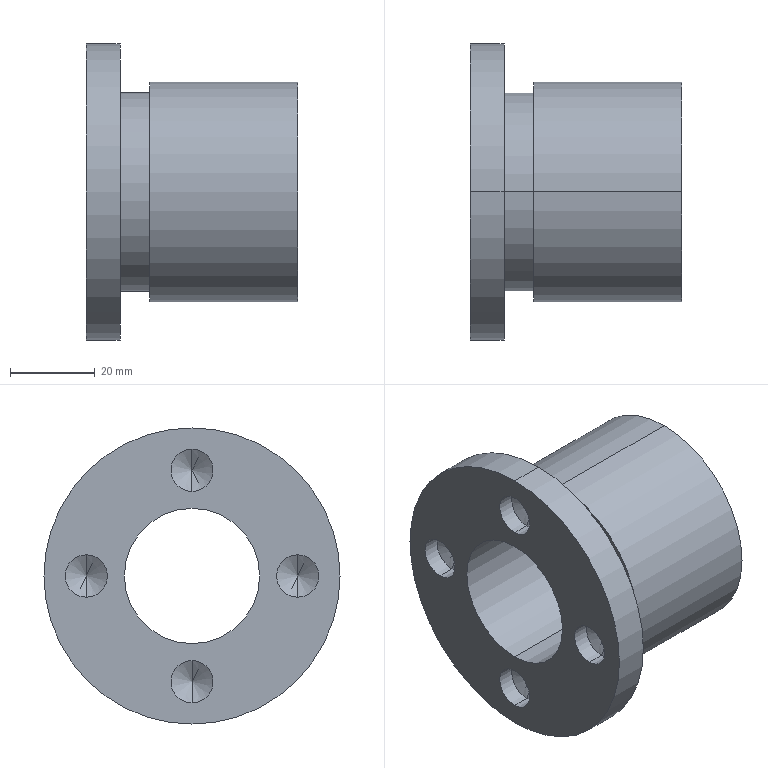Part | SolidWorks | features 3DProfileFeature 1, CirPattern 1, HoleWzd 1, Revolution 1 | 1 solid | 28 faces | box 50 x 70 x 70 mm | volume 75479 mm3 | cylinder 16 | cone 8 | plane 4 | commonest cylinder face diameters 10 x8 32 x2 47 x2 52 x2 70 x2
STEP:
#1=CARTESIAN_POINT('',(4.,0.,20.));
#2=VERTEX_POINT('',#1);
#3=CARTESIAN_POINT('',(4.,0.,30.));
#4=VERTEX_POINT('',#3);
#5=CARTESIAN_POINT('',(4.,0.,25.));
#6=DIRECTION('',(-1.,0.,0.));
#7=DIRECTION('',(0.,0.,1.));
#8=AXIS2_PLACEMENT_3D('',#5,#6,#7);
#9=CIRCLE('',#8,5.);
#10=EDGE_CURVE('',#2,#4,#9,.T.);
#11=ORIENTED_EDGE('',*,*,#10,.F.);
#12=CARTESIAN_POINT('',(0.,0.,20.));
#13=VERTEX_POINT('',#12);
#14=CARTESIAN_POINT('',(0.,0.,20.));
#15=DIRECTION('',(-1.,0.,0.));
#16=VECTOR('',#15,1000.);
#17=LINE('',#14,#16);
#18=EDGE_CURVE('',#2,#13,#17,.T.);
#19=ORIENTED_EDGE('',*,*,#18,.T.);
#20=CARTESIAN_POINT('',(0.,0.,30.));
#21=VERTEX_POINT('',#20);
#22=CARTESIAN_POINT('',(0.,0.,25.));
#23=DIRECTION('',(-1.,0.,0.));
#24=DIRECTION('',(0.,0.,1.));
#25=AXIS2_PLACEMENT_3D('',#22,#23,#24);
#26=CIRCLE('',#25,5.);
#27=EDGE_CURVE('',#13,#21,#26,.T.);
#28=ORIENTED_EDGE('',*,*,#27,.T.);
#29=CARTESIAN_POINT('',(0.,0.,30.));
#30=DIRECTION('',(-1.,0.,0.));
#31=VECTOR('',#30,1000.);
#32=LINE('',#29,#31);
#33=EDGE_CURVE('',#4,#21,#32,.T.);
#34=ORIENTED_EDGE('',*,*,#33,.F.);
#35=EDGE_LOOP('',(#11,#19,#28,#34));
#36=FACE_OUTER_BOUND('',#35,.T.);
#37=CARTESIAN_POINT('',(0.,0.,25.));
#38=DIRECTION('',(-1.,0.,0.));
#39=DIRECTION('',(0.,0.,1.));
#40=AXIS2_PLACEMENT_3D('',#37,#38,#39);
#41=CYLINDRICAL_SURFACE('',#40,5.);
#42=ADVANCED_FACE('',(#36),#41,.F.);
#43=CARTESIAN_POINT('',(7.004,0.,25.));
#44=VERTEX_POINT('',#43);
#45=CARTESIAN_POINT('',(4.,0.,30.));
#46=DIRECTION('',(-0.515,0.,0.8572));
#47=VECTOR('',#46,1000.);
#48=LINE('',#45,#47);
#49=EDGE_CURVE('',#44,#4,#48,.T.);
#50=ORIENTED_EDGE('',*,*,#49,.F.);
#51=CARTESIAN_POINT('',(4.,0.,20.));
#52=DIRECTION('',(-0.515,0.,-0.8572));
#53=VECTOR('',#52,1000.);
#54=LINE('',#51,#53);
#55=EDGE_CURVE('',#44,#2,#54,.T.);
#56=ORIENTED_EDGE('',*,*,#55,.T.);
#57=ORIENTED_EDGE('',*,*,#10,.T.);
#58=EDGE_LOOP('',(#50,#56,#57));
#59=FACE_OUTER_BOUND('',#58,.T.);
#60=CARTESIAN_POINT('',(4.,0.,25.));
#61=DIRECTION('',(-1.,0.,0.));
#62=DIRECTION('',(0.,0.,1.));
#63=AXIS2_PLACEMENT_3D('',#60,#61,#62);
#64=CONICAL_SURFACE('',#63,5.,1.03);
#65=ADVANCED_FACE('',(#59),#64,.F.);
#66=CARTESIAN_POINT('',(4.,-25.,-5.));
#67=VERTEX_POINT('',#66);
#68=CARTESIAN_POINT('',(4.,-25.,5.));
#69=VERTEX_POINT('',#68);
#70=CARTESIAN_POINT('',(4.,-25.,0.));
#71=DIRECTION('',(-1.,0.,0.));
#72=DIRECTION('',(0.,0.,1.));
#73=AXIS2_PLACEMENT_3D('',#70,#71,#72);
#74=CIRCLE('',#73,5.);
#75=EDGE_CURVE('',#67,#69,#74,.T.);
#76=ORIENTED_EDGE('',*,*,#75,.F.);
#77=CARTESIAN_POINT('',(0.,-25.,-5.));
#78=VERTEX_POINT('',#77);
#79=CARTESIAN_POINT('',(0.,-25.,-5.));
#80=DIRECTION('',(-1.,0.,0.));
#81=VECTOR('',#80,1000.);
#82=LINE('',#79,#81);
#83=EDGE_CURVE('',#67,#78,#82,.T.);
#84=ORIENTED_EDGE('',*,*,#83,.T.);
#85=CARTESIAN_POINT('',(0.,-25.,5.));
#86=VERTEX_POINT('',#85);
#87=CARTESIAN_POINT('',(0.,-25.,0.));
#88=DIRECTION('',(-1.,0.,0.));
#89=DIRECTION('',(0.,0.,1.));
#90=AXIS2_PLACEMENT_3D('',#87,#88,#89);
#91=CIRCLE('',#90,5.);
#92=EDGE_CURVE('',#78,#86,#91,.T.);
#93=ORIENTED_EDGE('',*,*,#92,.T.);
#94=CARTESIAN_POINT('',(0.,-25.,5.));
#95=DIRECTION('',(-1.,0.,0.));
#96=VECTOR('',#95,1000.);
#97=LINE('',#94,#96);
#98=EDGE_CURVE('',#69,#86,#97,.T.);
#99=ORIENTED_EDGE('',*,*,#98,.F.);
#100=EDGE_LOOP('',(#76,#84,#93,#99));
#101=FACE_OUTER_BOUND('',#100,.T.);
#102=CARTESIAN_POINT('',(0.,-25.,0.));
#103=DIRECTION('',(-1.,0.,0.));
#104=DIRECTION('',(0.,0.,1.));
#105=AXIS2_PLACEMENT_3D('',#102,#103,#104);
#106=CYLINDRICAL_SURFACE('',#105,5.);
#107=ADVANCED_FACE('',(#101),#106,.F.);
#108=CARTESIAN_POINT('',(7.004,-25.,0.));
#109=VERTEX_POINT('',#108);
#110=CARTESIAN_POINT('',(4.,-25.,5.));
#111=DIRECTION('',(-0.515,0.,0.8572));
#112=VECTOR('',#111,1000.);
#113=LINE('',#110,#112);
#114=EDGE_CURVE('',#109,#69,#113,.T.);
#115=ORIENTED_EDGE('',*,*,#114,.F.);
#116=CARTESIAN_POINT('',(4.,-25.,-5.));
#117=DIRECTION('',(-0.515,0.,-0.8572));
#118=VECTOR('',#117,1000.);
#119=LINE('',#116,#118);
#120=EDGE_CURVE('',#109,#67,#119,.T.);
#121=ORIENTED_EDGE('',*,*,#120,.T.);
#122=ORIENTED_EDGE('',*,*,#75,.T.);
#123=EDGE_LOOP('',(#115,#121,#122));
#124=FACE_OUTER_BOUND('',#123,.T.);
#125=CARTESIAN_POINT('',(4.,-25.,0.));
#126=DIRECTION('',(-1.,0.,0.));
#127=DIRECTION('',(0.,0.,1.));
#128=AXIS2_PLACEMENT_3D('',#125,#126,#127);
#129=CONICAL_SURFACE('',#128,5.,1.03);
#130=ADVANCED_FACE('',(#124),#129,.F.);
#131=CARTESIAN_POINT('',(4.,0.,-30.));
#132=VERTEX_POINT('',#131);
#133=CARTESIAN_POINT('',(4.,0.,-20.));
#134=VERTEX_POINT('',#133);
#135=CARTESIAN_POINT('',(4.,0.,-25.));
#136=DIRECTION('',(-1.,0.,0.));
#137=DIRECTION('',(0.,0.,1.));
#138=AXIS2_PLACEMENT_3D('',#135,#136,#137);
#139=CIRCLE('',#138,5.);
#140=EDGE_CURVE('',#132,#134,#139,.T.);
#141=ORIENTED_EDGE('',*,*,#140,.F.);
#142=CARTESIAN_POINT('',(0.,0.,-30.));
#143=VERTEX_POINT('',#142);
#144=CARTESIAN_POINT('',(0.,0.,-30.));
#145=DIRECTION('',(-1.,0.,0.));
#146=VECTOR('',#145,1000.);
#147=LINE('',#144,#146);
#148=EDGE_CURVE('',#132,#143,#147,.T.);
#149=ORIENTED_EDGE('',*,*,#148,.T.);
#150=CARTESIAN_POINT('',(0.,0.,-20.));
#151=VERTEX_POINT('',#150);
#152=CARTESIAN_POINT('',(0.,0.,-25.));
#153=DIRECTION('',(-1.,0.,0.));
#154=DIRECTION('',(0.,0.,1.));
#155=AXIS2_PLACEMENT_3D('',#152,#153,#154);
#156=CIRCLE('',#155,5.);
#157=EDGE_CURVE('',#143,#151,#156,.T.);
#158=ORIENTED_EDGE('',*,*,#157,.T.);
#159=CARTESIAN_POINT('',(0.,0.,-20.));
#160=DIRECTION('',(-1.,0.,0.));
#161=VECTOR('',#160,1000.);
#162=LINE('',#159,#161);
#163=EDGE_CURVE('',#134,#151,#162,.T.);
#164=ORIENTED_EDGE('',*,*,#163,.F.);
#165=EDGE_LOOP('',(#141,#149,#158,#164));
#166=FACE_OUTER_BOUND('',#165,.T.);
#167=CARTESIAN_POINT('',(0.,0.,-25.));
#168=DIRECTION('',(-1.,0.,0.));
#169=DIRECTION('',(0.,0.,1.));
#170=AXIS2_PLACEMENT_3D('',#167,#168,#169);
#171=CYLINDRICAL_SURFACE('',#170,5.);
#172=ADVANCED_FACE('',(#166),#171,.F.);
#173=CARTESIAN_POINT('',(7.004,0.,-25.));
#174=VERTEX_POINT('',#173);
#175=CARTESIAN_POINT('',(4.,0.,-20.));
#176=DIRECTION('',(-0.515,0.,0.8572));
#177=VECTOR('',#176,1000.);
#178=LINE('',#175,#177);
#179=EDGE_CURVE('',#174,#134,#178,.T.);
#180=ORIENTED_EDGE('',*,*,#179,.F.);
#181=CARTESIAN_POINT('',(4.,0.,-30.));
#182=DIRECTION('',(-0.515,0.,-0.8572));
#183=VECTOR('',#182,1000.);
#184=LINE('',#181,#183);
#185=EDGE_CURVE('',#174,#132,#184,.T.);
#186=ORIENTED_EDGE('',*,*,#185,.T.);
#187=ORIENTED_EDGE('',*,*,#140,.T.);
#188=EDGE_LOOP('',(#180,#186,#187));
#189=FACE_OUTER_BOUND('',#188,.T.);
#190=CARTESIAN_POINT('',(4.,0.,-25.));
#191=DIRECTION('',(-1.,0.,0.));
#192=DIRECTION('',(0.,0.,1.));
#193=AXIS2_PLACEMENT_3D('',#190,#191,#192);
#194=CONICAL_SURFACE('',#193,5.,1.03);
#195=ADVANCED_FACE('',(#189),#194,.F.);
#196=CARTESIAN_POINT('',(4.,25.,-5.));
#197=VERTEX_POINT('',#196);
#198=CARTESIAN_POINT('',(4.,25.,5.));
#199=VERTEX_POINT('',#198);
#200=CARTESIAN_POINT('',(4.,25.,0.));
#201=DIRECTION('',(-1.,0.,0.));
#202=DIRECTION('',(0.,0.,1.));
#203=AXIS2_PLACEMENT_3D('',#200,#201,#202);
#204=CIRCLE('',#203,5.);
#205=EDGE_CURVE('',#197,#199,#204,.T.);
#206=ORIENTED_EDGE('',*,*,#205,.F.);
#207=CARTESIAN_POINT('',(0.,25.,-5.));
#208=VERTEX_POINT('',#207);
#209=CARTESIAN_POINT('',(0.,25.,-5.));
#210=DIRECTION('',(-1.,0.,0.));
#211=VECTOR('',#210,1000.);
#212=LINE('',#209,#211);
#213=EDGE_CURVE('',#197,#208,#212,.T.);
#214=ORIENTED_EDGE('',*,*,#213,.T.);
#215=CARTESIAN_POINT('',(0.,25.,5.));
#216=VERTEX_POINT('',#215);
#217=CARTESIAN_POINT('',(0.,25.,0.));
#218=DIRECTION('',(-1.,0.,0.));
#219=DIRECTION('',(0.,0.,1.));
#220=AXIS2_PLACEMENT_3D('',#217,#218,#219);
#221=CIRCLE('',#220,5.);
#222=EDGE_CURVE('',#208,#216,#221,.T.);
#223=ORIENTED_EDGE('',*,*,#222,.T.);
#224=CARTESIAN_POINT('',(0.,25.,5.));
#225=DIRECTION('',(-1.,0.,0.));
#226=VECTOR('',#225,1000.);
#227=LINE('',#224,#226);
#228=EDGE_CURVE('',#199,#216,#227,.T.);
#229=ORIENTED_EDGE('',*,*,#228,.F.);
#230=EDGE_LOOP('',(#206,#214,#223,#229));
#231=FACE_OUTER_BOUND('',#230,.T.);
#232=CARTESIAN_POINT('',(0.,25.,0.));
#233=DIRECTION('',(-1.,0.,0.));
#234=DIRECTION('',(0.,0.,1.));
#235=AXIS2_PLACEMENT_3D('',#232,#233,#234);
#236=CYLINDRICAL_SURFACE('',#235,5.);
#237=ADVANCED_FACE('',(#231),#236,.F.);
#238=CARTESIAN_POINT('',(7.004,25.,0.));
#239=VERTEX_POINT('',#238);
#240=CARTESIAN_POINT('',(4.,25.,5.));
#241=DIRECTION('',(-0.515,0.,0.8572));
#242=VECTOR('',#241,1000.);
#243=LINE('',#240,#242);
#244=EDGE_CURVE('',#239,#199,#243,.T.);
#245=ORIENTED_EDGE('',*,*,#244,.F.);
#246=CARTESIAN_POINT('',(4.,25.,-5.));
#247=DIRECTION('',(-0.515,0.,-0.8572));
#248=VECTOR('',#247,1000.);
#249=LINE('',#246,#248);
#250=EDGE_CURVE('',#239,#197,#249,.T.);
#251=ORIENTED_EDGE('',*,*,#250,.T.);
#252=ORIENTED_EDGE('',*,*,#205,.T.);
#253=EDGE_LOOP('',(#245,#251,#252));
#254=FACE_OUTER_BOUND('',#253,.T.);
#255=CARTESIAN_POINT('',(4.,25.,0.));
#256=DIRECTION('',(-1.,0.,0.));
#257=DIRECTION('',(0.,0.,1.));
#258=AXIS2_PLACEMENT_3D('',#255,#256,#257);
#259=CONICAL_SURFACE('',#258,5.,1.03);
#260=ADVANCED_FACE('',(#254),#259,.F.);
#261=CARTESIAN_POINT('',(50.,0.,26.));
#262=VERTEX_POINT('',#261);
#263=CARTESIAN_POINT('',(50.,0.,-26.));
#264=VERTEX_POINT('',#263);
#265=CARTESIAN_POINT('',(50.,0.,0.));
#266=DIRECTION('',(-1.,0.,0.));
#267=DIRECTION('',(0.,0.,1.));
#268=AXIS2_PLACEMENT_3D('',#265,#266,#267);
#269=CIRCLE('',#268,26.);
#270=EDGE_CURVE('',#262,#264,#269,.T.);
#271=ORIENTED_EDGE('',*,*,#270,.T.);
#272=CARTESIAN_POINT('',(15.,0.,-26.));
#273=VERTEX_POINT('',#272);
#274=CARTESIAN_POINT('',(0.,0.,-26.));
#275=DIRECTION('',(-1.,0.,0.));
#276=VECTOR('',#275,1000.);
#277=LINE('',#274,#276);
#278=EDGE_CURVE('',#264,#273,#277,.T.);
#279=ORIENTED_EDGE('',*,*,#278,.T.);
#280=CARTESIAN_POINT('',(15.,0.,26.));
#281=VERTEX_POINT('',#280);
#282=CARTESIAN_POINT('',(15.,0.,0.));
#283=DIRECTION('',(-1.,0.,0.));
#284=DIRECTION('',(0.,0.,1.));
#285=AXIS2_PLACEMENT_3D('',#282,#283,#284);
#286=CIRCLE('',#285,26.);
#287=EDGE_CURVE('',#281,#273,#286,.T.);
#288=ORIENTED_EDGE('',*,*,#287,.F.);
#289=CARTESIAN_POINT('',(0.,0.,26.));
#290=DIRECTION('',(-1.,0.,0.));
#291=VECTOR('',#290,1000.);
#292=LINE('',#289,#291);
#293=EDGE_CURVE('',#262,#281,#292,.T.);
#294=ORIENTED_EDGE('',*,*,#293,.F.);
#295=EDGE_LOOP('',(#271,#279,#288,#294));
#296=FACE_OUTER_BOUND('',#295,.T.);
#297=CARTESIAN_POINT('',(0.,0.,0.));
#298=DIRECTION('',(-1.,0.,0.));
#299=DIRECTION('',(0.,0.,1.));
#300=AXIS2_PLACEMENT_3D('',#297,#298,#299);
#301=CYLINDRICAL_SURFACE('',#300,26.);
#302=ADVANCED_FACE('',(#296),#301,.T.);
#303=CARTESIAN_POINT('',(15.,0.,23.5));
#304=VERTEX_POINT('',#303);
#305=CARTESIAN_POINT('',(15.,0.,-23.5));
#306=VERTEX_POINT('',#305);
#307=CARTESIAN_POINT('',(15.,0.,0.));
#308=DIRECTION('',(-1.,0.,0.));
#309=DIRECTION('',(0.,0.,1.));
#310=AXIS2_PLACEMENT_3D('',#307,#308,#309);
#311=CIRCLE('',#310,23.5);
#312=EDGE_CURVE('',#304,#306,#311,.T.);
#313=ORIENTED_EDGE('',*,*,#312,.T.);
#314=CARTESIAN_POINT('',(8.,0.,-23.5));
#315=VERTEX_POINT('',#314);
#316=CARTESIAN_POINT('',(0.,0.,-23.5));
#317=DIRECTION('',(-1.,0.,0.));
#318=VECTOR('',#317,1000.);
#319=LINE('',#316,#318);
#320=EDGE_CURVE('',#306,#315,#319,.T.);
#321=ORIENTED_EDGE('',*,*,#320,.T.);
#322=CARTESIAN_POINT('',(8.,0.,23.5));
#323=VERTEX_POINT('',#322);
#324=CARTESIAN_POINT('',(8.,0.,0.));
#325=DIRECTION('',(-1.,0.,0.));
#326=DIRECTION('',(0.,0.,1.));
#327=AXIS2_PLACEMENT_3D('',#324,#325,#326);
#328=CIRCLE('',#327,23.5);
#329=EDGE_CURVE('',#323,#315,#328,.T.);
#330=ORIENTED_EDGE('',*,*,#329,.F.);
#331=CARTESIAN_POINT('',(0.,0.,23.5));
#332=DIRECTION('',(-1.,0.,0.));
#333=VECTOR('',#332,1000.);
#334=LINE('',#331,#333);
#335=EDGE_CURVE('',#304,#323,#334,.T.);
#336=ORIENTED_EDGE('',*,*,#335,.F.);
#337=EDGE_LOOP('',(#313,#321,#330,#336));
#338=FACE_OUTER_BOUND('',#337,.T.);
#339=CARTESIAN_POINT('',(0.,0.,0.));
#340=DIRECTION('',(-1.,0.,0.));
#341=DIRECTION('',(0.,0.,1.));
#342=AXIS2_PLACEMENT_3D('',#339,#340,#341);
#343=CYLINDRICAL_SURFACE('',#342,23.5);
#344=ADVANCED_FACE('',(#338),#343,.T.);
#345=CARTESIAN_POINT('',(8.,0.,35.));
#346=VERTEX_POINT('',#345);
#347=CARTESIAN_POINT('',(8.,0.,-35.));
#348=VERTEX_POINT('',#347);
#349=CARTESIAN_POINT('',(8.,0.,0.));
#350=DIRECTION('',(-1.,0.,0.));
#351=DIRECTION('',(0.,0.,1.));
#352=AXIS2_PLACEMENT_3D('',#349,#350,#351);
#353=CIRCLE('',#352,35.);
#354=EDGE_CURVE('',#346,#348,#353,.T.);
#355=ORIENTED_EDGE('',*,*,#354,.T.);
#356=CARTESIAN_POINT('',(0.,0.,-35.));
#357=VERTEX_POINT('',#356);
#358=CARTESIAN_POINT('',(0.,0.,-35.));
#359=DIRECTION('',(-1.,0.,0.));
#360=VECTOR('',#359,1000.);
#361=LINE('',#358,#360);
#362=EDGE_CURVE('',#348,#357,#361,.T.);
#363=ORIENTED_EDGE('',*,*,#362,.T.);
#364=CARTESIAN_POINT('',(0.,0.,35.));
#365=VERTEX_POINT('',#364);
#366=CARTESIAN_POINT('',(0.,0.,0.));
#367=DIRECTION('',(-1.,0.,0.));
#368=DIRECTION('',(0.,0.,1.));
#369=AXIS2_PLACEMENT_3D('',#366,#367,#368);
#370=CIRCLE('',#369,35.);
#371=EDGE_CURVE('',#365,#357,#370,.T.);
#372=ORIENTED_EDGE('',*,*,#371,.F.);
#373=CARTESIAN_POINT('',(0.,0.,35.));
#374=DIRECTION('',(-1.,0.,0.));
#375=VECTOR('',#374,1000.);
#376=LINE('',#373,#375);
#377=EDGE_CURVE('',#346,#365,#376,.T.);
#378=ORIENTED_EDGE('',*,*,#377,.F.);
#379=EDGE_LOOP('',(#355,#363,#372,#378));
#380=FACE_OUTER_BOUND('',#379,.T.);
#381=CARTESIAN_POINT('',(0.,0.,0.));
#382=DIRECTION('',(-1.,0.,0.));
#383=DIRECTION('',(0.,0.,1.));
#384=AXIS2_PLACEMENT_3D('',#381,#382,#383);
#385=CYLINDRICAL_SURFACE('',#384,35.);
#386=ADVANCED_FACE('',(#380),#385,.T.);
#387=CARTESIAN_POINT('',(50.,0.,-16.));
#388=VERTEX_POINT('',#387);
#389=CARTESIAN_POINT('',(50.,0.,16.));
#390=VERTEX_POINT('',#389);
#391=CARTESIAN_POINT('',(50.,0.,0.));
#392=DIRECTION('',(-1.,0.,0.));
#393=DIRECTION('',(0.,0.,1.));
#394=AXIS2_PLACEMENT_3D('',#391,#392,#393);
#395=CIRCLE('',#394,16.);
#396=EDGE_CURVE('',#388,#390,#395,.T.);
#397=ORIENTED_EDGE('',*,*,#396,.F.);
#398=CARTESIAN_POINT('',(0.,0.,-16.));
#399=VERTEX_POINT('',#398);
#400=CARTESIAN_POINT('',(0.,0.,-16.));
#401=DIRECTION('',(-1.,0.,0.));
#402=VECTOR('',#401,1000.);
#403=LINE('',#400,#402);
#404=EDGE_CURVE('',#388,#399,#403,.T.);
#405=ORIENTED_EDGE('',*,*,#404,.T.);
#406=CARTESIAN_POINT('',(0.,0.,16.));
#407=VERTEX_POINT('',#406);
#408=CARTESIAN_POINT('',(0.,0.,0.));
#409=DIRECTION('',(-1.,0.,0.));
#410=DIRECTION('',(0.,0.,1.));
#411=AXIS2_PLACEMENT_3D('',#408,#409,#410);
#412=CIRCLE('',#411,16.);
#413=EDGE_CURVE('',#399,#407,#412,.T.);
#414=ORIENTED_EDGE('',*,*,#413,.T.);
#415=CARTESIAN_POINT('',(0.,0.,16.));
#416=DIRECTION('',(-1.,0.,0.));
#417=VECTOR('',#416,1000.);
#418=LINE('',#415,#417);
#419=EDGE_CURVE('',#390,#407,#418,.T.);
#420=ORIENTED_EDGE('',*,*,#419,.F.);
#421=EDGE_LOOP('',(#397,#405,#414,#420));
#422=FACE_OUTER_BOUND('',#421,.T.);
#423=CARTESIAN_POINT('',(0.,0.,0.));
#424=DIRECTION('',(-1.,0.,0.));
#425=DIRECTION('',(0.,0.,1.));
#426=AXIS2_PLACEMENT_3D('',#423,#424,#425);
#427=CYLINDRICAL_SURFACE('',#426,16.);
#428=ADVANCED_FACE('',(#422),#427,.F.);
#429=ORIENTED_EDGE('',*,*,#404,.F.);
#430=CARTESIAN_POINT('',(50.,0.,0.));
#431=DIRECTION('',(-1.,0.,0.));
#432=DIRECTION('',(0.,0.,1.));
#433=AXIS2_PLACEMENT_3D('',#430,#431,#432);
#434=CIRCLE('',#433,16.);
#435=EDGE_CURVE('',#390,#388,#434,.T.);
#436=ORIENTED_EDGE('',*,*,#435,.F.);
#437=ORIENTED_EDGE('',*,*,#419,.T.);
#438=CARTESIAN_POINT('',(0.,0.,0.));
#439=DIRECTION('',(-1.,0.,0.));
#440=DIRECTION('',(0.,0.,1.));
#441=AXIS2_PLACEMENT_3D('',#438,#439,#440);
#442=CIRCLE('',#441,16.);
#443=EDGE_CURVE('',#407,#399,#442,.T.);
#444=ORIENTED_EDGE('',*,*,#443,.T.);
#445=EDGE_LOOP('',(#429,#436,#437,#444));
#446=FACE_OUTER_BOUND('',#445,.T.);
#447=CARTESIAN_POINT('',(0.,0.,0.));
#448=DIRECTION('',(-1.,0.,0.));
#449=DIRECTION('',(0.,0.,1.));
#450=AXIS2_PLACEMENT_3D('',#447,#448,#449);
#451=CYLINDRICAL_SURFACE('',#450,16.);
#452=ADVANCED_FACE('',(#446),#451,.F.);
#453=CARTESIAN_POINT('',(0.,0.,25.));
#454=DIRECTION('',(-1.,0.,0.));
#455=DIRECTION('',(0.,0.,1.));
#456=AXIS2_PLACEMENT_3D('',#453,#454,#455);
#457=CIRCLE('',#456,5.);
#458=EDGE_CURVE('',#21,#13,#457,.T.);
#459=ORIENTED_EDGE('',*,*,#458,.F.);
#460=ORIENTED_EDGE('',*,*,#27,.F.);
#461=EDGE_LOOP('',(#459,#460));
#462=FACE_BOUND('',#461,.T.);
#463=CARTESIAN_POINT('',(0.,-25.,0.));
#464=DIRECTION('',(-1.,0.,0.));
#465=DIRECTION('',(0.,0.,1.));
#466=AXIS2_PLACEMENT_3D('',#463,#464,#465);
#467=CIRCLE('',#466,5.);
#468=EDGE_CURVE('',#86,#78,#467,.T.);
#469=ORIENTED_EDGE('',*,*,#468,.F.);
#470=ORIENTED_EDGE('',*,*,#92,.F.);
#471=EDGE_LOOP('',(#469,#470));
#472=FACE_BOUND('',#471,.T.);
#473=CARTESIAN_POINT('',(0.,0.,-25.));
#474=DIRECTION('',(-1.,0.,0.));
#475=DIRECTION('',(0.,0.,1.));
#476=AXIS2_PLACEMENT_3D('',#473,#474,#475);
#477=CIRCLE('',#476,5.);
#478=EDGE_CURVE('',#151,#143,#477,.T.);
#479=ORIENTED_EDGE('',*,*,#478,.F.);
#480=ORIENTED_EDGE('',*,*,#157,.F.);
#481=EDGE_LOOP('',(#479,#480));
#482=FACE_BOUND('',#481,.T.);
#483=CARTESIAN_POINT('',(0.,25.,0.));
#484=DIRECTION('',(-1.,0.,0.));
#485=DIRECTION('',(0.,0.,1.));
#486=AXIS2_PLACEMENT_3D('',#483,#484,#485);
#487=CIRCLE('',#486,5.);
#488=EDGE_CURVE('',#216,#208,#487,.T.);
#489=ORIENTED_EDGE('',*,*,#488,.F.);
#490=ORIENTED_EDGE('',*,*,#222,.F.);
#491=EDGE_LOOP('',(#489,#490));
#492=FACE_BOUND('',#491,.T.);
#493=ORIENTED_EDGE('',*,*,#443,.F.);
#494=ORIENTED_EDGE('',*,*,#413,.F.);
#495=EDGE_LOOP('',(#493,#494));
#496=FACE_BOUND('',#495,.T.);
#497=ORIENTED_EDGE('',*,*,#371,.T.);
#498=CARTESIAN_POINT('',(0.,0.,0.));
#499=DIRECTION('',(-1.,0.,0.));
#500=DIRECTION('',(0.,0.,1.));
#501=AXIS2_PLACEMENT_3D('',#498,#499,#500);
#502=CIRCLE('',#501,35.);
#503=EDGE_CURVE('',#357,#365,#502,.T.);
#504=ORIENTED_EDGE('',*,*,#503,.T.);
#505=EDGE_LOOP('',(#497,#504));
#506=FACE_OUTER_BOUND('',#505,.T.);
#507=CARTESIAN_POINT('',(0.,16.,0.));
#508=DIRECTION('',(1.,0.,0.));
#509=DIRECTION('',(0.,0.,-1.));
#510=AXIS2_PLACEMENT_3D('',#507,#508,#509);
#511=PLANE('',#510);
#512=ADVANCED_FACE('',(#462,#472,#482,#492,#496,#506),#511,.F.);
#513=ORIENTED_EDGE('',*,*,#362,.F.);
#514=CARTESIAN_POINT('',(8.,0.,0.));
#515=DIRECTION('',(-1.,0.,0.));
#516=DIRECTION('',(0.,0.,1.));
#517=AXIS2_PLACEMENT_3D('',#514,#515,#516);
#518=CIRCLE('',#517,35.);
#519=EDGE_CURVE('',#348,#346,#518,.T.);
#520=ORIENTED_EDGE('',*,*,#519,.T.);
#521=ORIENTED_EDGE('',*,*,#377,.T.);
#522=ORIENTED_EDGE('',*,*,#503,.F.);
#523=EDGE_LOOP('',(#513,#520,#521,#522));
#524=FACE_OUTER_BOUND('',#523,.T.);
#525=CARTESIAN_POINT('',(0.,0.,0.));
#526=DIRECTION('',(-1.,0.,0.));
#527=DIRECTION('',(0.,0.,1.));
#528=AXIS2_PLACEMENT_3D('',#525,#526,#527);
#529=CYLINDRICAL_SURFACE('',#528,35.);
#530=ADVANCED_FACE('',(#524),#529,.T.);
#531=ORIENTED_EDGE('',*,*,#354,.F.);
#532=ORIENTED_EDGE('',*,*,#519,.F.);
#533=EDGE_LOOP('',(#531,#532));
#534=FACE_OUTER_BOUND('',#533,.T.);
#535=ORIENTED_EDGE('',*,*,#329,.T.);
#536=CARTESIAN_POINT('',(8.,0.,0.));
#537=DIRECTION('',(-1.,0.,0.));
#538=DIRECTION('',(0.,0.,1.));
#539=AXIS2_PLACEMENT_3D('',#536,#537,#538);
#540=CIRCLE('',#539,23.5);
#541=EDGE_CURVE('',#315,#323,#540,.T.);
#542=ORIENTED_EDGE('',*,*,#541,.T.);
#543=EDGE_LOOP('',(#535,#542));
#544=FACE_BOUND('',#543,.T.);
#545=CARTESIAN_POINT('',(8.,35.,0.));
#546=DIRECTION('',(-1.,0.,0.));
#547=DIRECTION('',(0.,0.,1.));
#548=AXIS2_PLACEMENT_3D('',#545,#546,#547);
#549=PLANE('',#548);
#550=ADVANCED_FACE('',(#534,#544),#549,.F.);
#551=ORIENTED_EDGE('',*,*,#320,.F.);
#552=CARTESIAN_POINT('',(15.,0.,0.));
#553=DIRECTION('',(-1.,0.,0.));
#554=DIRECTION('',(0.,0.,1.));
#555=AXIS2_PLACEMENT_3D('',#552,#553,#554);
#556=CIRCLE('',#555,23.5);
#557=EDGE_CURVE('',#306,#304,#556,.T.);
#558=ORIENTED_EDGE('',*,*,#557,.T.);
#559=ORIENTED_EDGE('',*,*,#335,.T.);
#560=ORIENTED_EDGE('',*,*,#541,.F.);
#561=EDGE_LOOP('',(#551,#558,#559,#560));
#562=FACE_OUTER_BOUND('',#561,.T.);
#563=CARTESIAN_POINT('',(0.,0.,0.));
#564=DIRECTION('',(-1.,0.,0.));
#565=DIRECTION('',(0.,0.,1.));
#566=AXIS2_PLACEMENT_3D('',#563,#564,#565);
#567=CYLINDRICAL_SURFACE('',#566,23.5);
#568=ADVANCED_FACE('',(#562),#567,.T.);
#569=ORIENTED_EDGE('',*,*,#312,.F.);
#570=ORIENTED_EDGE('',*,*,#557,.F.);
#571=EDGE_LOOP('',(#569,#570));
#572=FACE_BOUND('',#571,.T.);
#573=ORIENTED_EDGE('',*,*,#287,.T.);
#574=CARTESIAN_POINT('',(15.,0.,0.));
#575=DIRECTION('',(-1.,0.,0.));
#576=DIRECTION('',(0.,0.,1.));
#577=AXIS2_PLACEMENT_3D('',#574,#575,#576);
#578=CIRCLE('',#577,26.);
#579=EDGE_CURVE('',#273,#281,#578,.T.);
#580=ORIENTED_EDGE('',*,*,#579,.T.);
#581=EDGE_LOOP('',(#573,#580));
#582=FACE_OUTER_BOUND('',#581,.T.);
#583=CARTESIAN_POINT('',(15.,23.5,0.));
#584=DIRECTION('',(1.,0.,0.));
#585=DIRECTION('',(0.,0.,-1.));
#586=AXIS2_PLACEMENT_3D('',#583,#584,#585);
#587=PLANE('',#586);
#588=ADVANCED_FACE('',(#572,#582),#587,.F.);
#589=ORIENTED_EDGE('',*,*,#278,.F.);
#590=CARTESIAN_POINT('',(50.,0.,0.));
#591=DIRECTION('',(-1.,0.,0.));
#592=DIRECTION('',(0.,0.,1.));
#593=AXIS2_PLACEMENT_3D('',#590,#591,#592);
#594=CIRCLE('',#593,26.);
#595=EDGE_CURVE('',#264,#262,#594,.T.);
#596=ORIENTED_EDGE('',*,*,#595,.T.);
#597=ORIENTED_EDGE('',*,*,#293,.T.);
#598=ORIENTED_EDGE('',*,*,#579,.F.);
#599=EDGE_LOOP('',(#589,#596,#597,#598));
#600=FACE_OUTER_BOUND('',#599,.T.);
#601=CARTESIAN_POINT('',(0.,0.,0.));
#602=DIRECTION('',(-1.,0.,0.));
#603=DIRECTION('',(0.,0.,1.));
#604=AXIS2_PLACEMENT_3D('',#601,#602,#603);
#605=CYLINDRICAL_SURFACE('',#604,26.);
#606=ADVANCED_FACE('',(#600),#605,.T.);
#607=ORIENTED_EDGE('',*,*,#270,.F.);
#608=ORIENTED_EDGE('',*,*,#595,.F.);
#609=EDGE_LOOP('',(#607,#608));
#610=FACE_OUTER_BOUND('',#609,.T.);
#611=ORIENTED_EDGE('',*,*,#435,.T.);
#612=ORIENTED_EDGE('',*,*,#396,.T.);
#613=EDGE_LOOP('',(#611,#612));
#614=FACE_BOUND('',#613,.T.);
#615=CARTESIAN_POINT('',(50.,26.,0.));
#616=DIRECTION('',(-1.,0.,0.));
#617=DIRECTION('',(0.,0.,1.));
#618=AXIS2_PLACEMENT_3D('',#615,#616,#617);
#619=PLANE('',#618);
#620=ADVANCED_FACE('',(#610,#614),#619,.F.);
#621=ORIENTED_EDGE('',*,*,#250,.F.);
#622=ORIENTED_EDGE('',*,*,#244,.T.);
#623=CARTESIAN_POINT('',(4.,25.,0.));
#624=DIRECTION('',(-1.,0.,0.));
#625=DIRECTION('',(0.,0.,1.));
#626=AXIS2_PLACEMENT_3D('',#623,#624,#625);
#627=CIRCLE('',#626,5.);
#628=EDGE_CURVE('',#199,#197,#627,.T.);
#629=ORIENTED_EDGE('',*,*,#628,.T.);
#630=EDGE_LOOP('',(#621,#622,#629));
#631=FACE_OUTER_BOUND('',#630,.T.);
#632=CARTESIAN_POINT('',(4.,25.,0.));
#633=DIRECTION('',(-1.,0.,0.));
#634=DIRECTION('',(0.,0.,1.));
#635=AXIS2_PLACEMENT_3D('',#632,#633,#634);
#636=CONICAL_SURFACE('',#635,5.,1.03);
#637=ADVANCED_FACE('',(#631),#636,.F.);
#638=ORIENTED_EDGE('',*,*,#213,.F.);
#639=ORIENTED_EDGE('',*,*,#628,.F.);
#640=ORIENTED_EDGE('',*,*,#228,.T.);
#641=ORIENTED_EDGE('',*,*,#488,.T.);
#642=EDGE_LOOP('',(#638,#639,#640,#641));
#643=FACE_OUTER_BOUND('',#642,.T.);
#644=CARTESIAN_POINT('',(0.,25.,0.));
#645=DIRECTION('',(-1.,0.,0.));
#646=DIRECTION('',(0.,0.,1.));
#647=AXIS2_PLACEMENT_3D('',#644,#645,#646);
#648=CYLINDRICAL_SURFACE('',#647,5.);
#649=ADVANCED_FACE('',(#643),#648,.F.);
#650=ORIENTED_EDGE('',*,*,#185,.F.);
#651=ORIENTED_EDGE('',*,*,#179,.T.);
#652=CARTESIAN_POINT('',(4.,0.,-25.));
#653=DIRECTION('',(-1.,0.,0.));
#654=DIRECTION('',(0.,0.,1.));
#655=AXIS2_PLACEMENT_3D('',#652,#653,#654);
#656=CIRCLE('',#655,5.);
#657=EDGE_CURVE('',#134,#132,#656,.T.);
#658=ORIENTED_EDGE('',*,*,#657,.T.);
#659=EDGE_LOOP('',(#650,#651,#658));
#660=FACE_OUTER_BOUND('',#659,.T.);
#661=CARTESIAN_POINT('',(4.,0.,-25.));
#662=DIRECTION('',(-1.,0.,0.));
#663=DIRECTION('',(0.,0.,1.));
#664=AXIS2_PLACEMENT_3D('',#661,#662,#663);
#665=CONICAL_SURFACE('',#664,5.,1.03);
#666=ADVANCED_FACE('',(#660),#665,.F.);
#667=ORIENTED_EDGE('',*,*,#148,.F.);
#668=ORIENTED_EDGE('',*,*,#657,.F.);
#669=ORIENTED_EDGE('',*,*,#163,.T.);
#670=ORIENTED_EDGE('',*,*,#478,.T.);
#671=EDGE_LOOP('',(#667,#668,#669,#670));
#672=FACE_OUTER_BOUND('',#671,.T.);
#673=CARTESIAN_POINT('',(0.,0.,-25.));
#674=DIRECTION('',(-1.,0.,0.));
#675=DIRECTION('',(0.,0.,1.));
#676=AXIS2_PLACEMENT_3D('',#673,#674,#675);
#677=CYLINDRICAL_SURFACE('',#676,5.);
#678=ADVANCED_FACE('',(#672),#677,.F.);
#679=ORIENTED_EDGE('',*,*,#120,.F.);
#680=ORIENTED_EDGE('',*,*,#114,.T.);
#681=CARTESIAN_POINT('',(4.,-25.,0.));
#682=DIRECTION('',(-1.,0.,0.));
#683=DIRECTION('',(0.,0.,1.));
#684=AXIS2_PLACEMENT_3D('',#681,#682,#683);
#685=CIRCLE('',#684,5.);
#686=EDGE_CURVE('',#69,#67,#685,.T.);
#687=ORIENTED_EDGE('',*,*,#686,.T.);
#688=EDGE_LOOP('',(#679,#680,#687));
#689=FACE_OUTER_BOUND('',#688,.T.);
#690=CARTESIAN_POINT('',(4.,-25.,0.));
#691=DIRECTION('',(-1.,0.,0.));
#692=DIRECTION('',(0.,0.,1.));
#693=AXIS2_PLACEMENT_3D('',#690,#691,#692);
#694=CONICAL_SURFACE('',#693,5.,1.03);
#695=ADVANCED_FACE('',(#689),#694,.F.);
#696=ORIENTED_EDGE('',*,*,#83,.F.);
#697=ORIENTED_EDGE('',*,*,#686,.F.);
#698=ORIENTED_EDGE('',*,*,#98,.T.);
#699=ORIENTED_EDGE('',*,*,#468,.T.);
#700=EDGE_LOOP('',(#696,#697,#698,#699));
#701=FACE_OUTER_BOUND('',#700,.T.);
#702=CARTESIAN_POINT('',(0.,-25.,0.));
#703=DIRECTION('',(-1.,0.,0.));
#704=DIRECTION('',(0.,0.,1.));
#705=AXIS2_PLACEMENT_3D('',#702,#703,#704);
#706=CYLINDRICAL_SURFACE('',#705,5.);
#707=ADVANCED_FACE('',(#701),#706,.F.);
#708=ORIENTED_EDGE('',*,*,#55,.F.);
#709=ORIENTED_EDGE('',*,*,#49,.T.);
#710=CARTESIAN_POINT('',(4.,0.,25.));
#711=DIRECTION('',(-1.,0.,0.));
#712=DIRECTION('',(0.,0.,1.));
#713=AXIS2_PLACEMENT_3D('',#710,#711,#712);
#714=CIRCLE('',#713,5.);
#715=EDGE_CURVE('',#4,#2,#714,.T.);
#716=ORIENTED_EDGE('',*,*,#715,.T.);
#717=EDGE_LOOP('',(#708,#709,#716));
#718=FACE_OUTER_BOUND('',#717,.T.);
#719=CARTESIAN_POINT('',(4.,0.,25.));
#720=DIRECTION('',(-1.,0.,0.));
#721=DIRECTION('',(0.,0.,1.));
#722=AXIS2_PLACEMENT_3D('',#719,#720,#721);
#723=CONICAL_SURFACE('',#722,5.,1.03);
#724=ADVANCED_FACE('',(#718),#723,.F.);
#725=ORIENTED_EDGE('',*,*,#18,.F.);
#726=ORIENTED_EDGE('',*,*,#715,.F.);
#727=ORIENTED_EDGE('',*,*,#33,.T.);
#728=ORIENTED_EDGE('',*,*,#458,.T.);
#729=EDGE_LOOP('',(#725,#726,#727,#728));
#730=FACE_OUTER_BOUND('',#729,.T.);
#731=CARTESIAN_POINT('',(0.,0.,25.));
#732=DIRECTION('',(-1.,0.,0.));
#733=DIRECTION('',(0.,0.,1.));
#734=AXIS2_PLACEMENT_3D('',#731,#732,#733);
#735=CYLINDRICAL_SURFACE('',#734,5.);
#736=ADVANCED_FACE('',(#730),#735,.F.);
#737=CLOSED_SHELL('',(#42,#65,#107,#130,#172,#195,#237,#260,#302,#344,#386,#428,#452,#512,#530,#550,#568,#588,#606,#620,#637,#649,#666,#678,#695,#707,#724,#736));
#738=MANIFOLD_SOLID_BREP('',#737);
#739=CARTESIAN_POINT('',(0.,0.,0.));
#740=DIRECTION('',(0.,0.,1.));
#741=DIRECTION('',(1.,0.,0.));
#742=AXIS2_PLACEMENT_3D('',#739,#740,#741);
#743=(LENGTH_UNIT()NAMED_UNIT(*)SI_UNIT(.MILLI.,.METRE.));
#744=UNCERTAINTY_MEASURE_WITH_UNIT(LENGTH_MEASURE(0.00001),#743,'','');
#745=(NAMED_UNIT(*)PLANE_ANGLE_UNIT()SI_UNIT($,.RADIAN.));
#746=(NAMED_UNIT(*)SI_UNIT($,.STERADIAN.)SOLID_ANGLE_UNIT());
#747=(GEOMETRIC_REPRESENTATION_CONTEXT(3)GLOBAL_UNCERTAINTY_ASSIGNED_CONTEXT((#744))GLOBAL_UNIT_ASSIGNED_CONTEXT((#743,#745,#746))REPRESENTATION_CONTEXT('',''));
#748=ADVANCED_BREP_SHAPE_REPRESENTATION('',(#738,#742),#747);